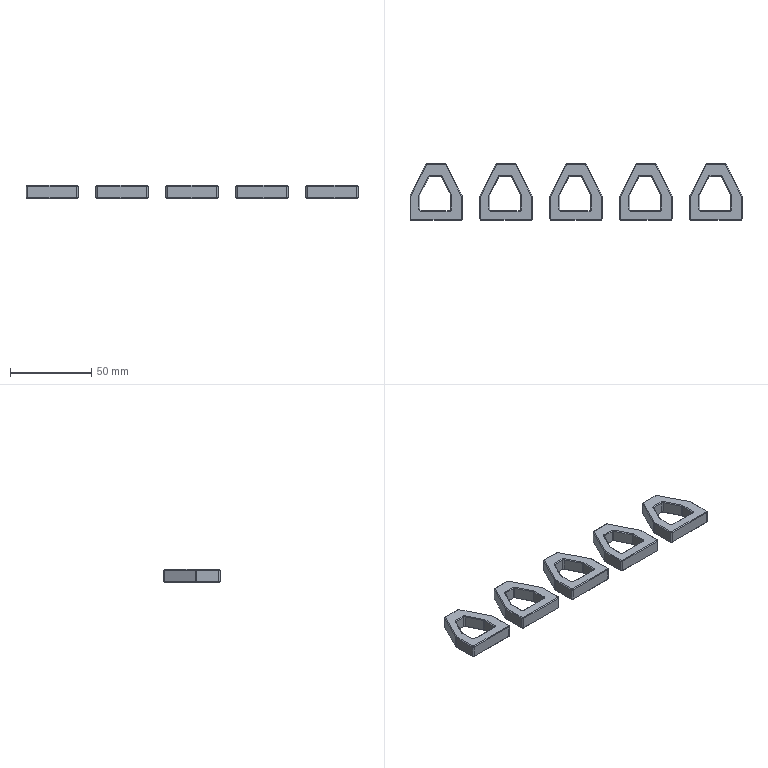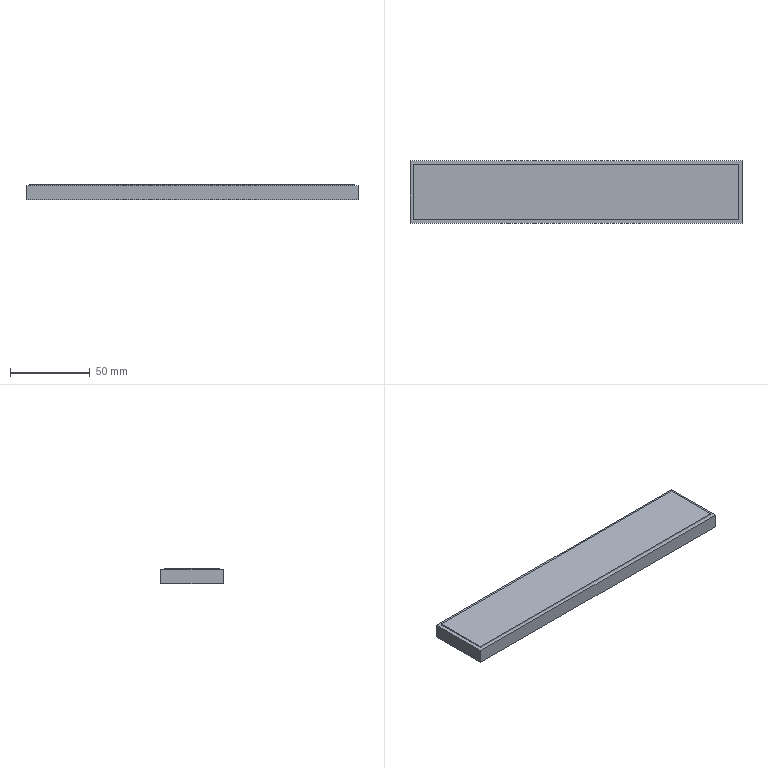CAM job | NX | 3-axis milling | part box 204 x 35 x 8 mm | stock box 208 x 39 x 10 mm
Tools:
number,name,description,diameter,corner_radius,flute_length,length,flutes
19,D80,Milling Tool-5 Parameters,80.0,0.0,50.0,75.0,2
15,D10,Milling Tool-5 Parameters,10.0,0.0,50.0,75.0,2
14,D10JING,Milling Tool-5 Parameters,10.0,0.0,50.0,75.0,2
11,D4,Milling Tool-5 Parameters,4.0,0.0,50.0,75.0,2
17,D3,Milling Tool-5 Parameters,3.0,0.0,50.0,75.0,2
16,D2,Milling Tool-5 Parameters,2.0,0.0,50.0,75.0,2
1,D6A45,Milling Tool-5 Parameters,6.0,0.0,50.0,75.0,2
Operations:
program,operation,operation_type,tool,method,geometry_group,spindle_rpm,surface_speed,feed_per_tooth,feed_cut,feed_plunge,cut_length_mm,path_length_mm,cut_time_min,machine_time_min
1,FLOOR_WALL,VolumeBased25DMillingOperation,D80,METHOD,A,6500.0,1633.0,0.1154,1500.0,100.0,300.0,354.0,0.2,0.2054
1,ZLEVEL_PROFILE_COPY_1,ZLevelMilling,D10,METHOD,A,9500.0,298.0,0.1842,3500.0,1000.0,8731.767,10477.213,2.836,3.01
1,PLANAR_PROFILE,PlanarMilling,D10,METHOD,A,9500.0,298.0,0.1842,3500.0,100.0,2440.0,5132.0,0.6971,0.9663
1,ZLEVEL_PROFILE_COPY_1_COPY,ZLevelMilling,D10JING,METHOD,A,9500.0,298.0,0.0632,1200.0,1000.0,967.776,2493.494,0.8107,0.9633
1,ZLEVEL_PROFILE_COPY_1_COPY_1,ZLevelMilling,D4,METHOD,A,9500.0,298.0,0.0947,1800.0,1000.0,3024.927,7224.257,1.863,2.282
1,HOLE_MILLING,CylinderMilling,D3,METHOD,A,9500.0,89.0,0.0605,1150.0,100.0,1287.723,2989.856,1.12,1.29
1,ZLEVEL_PROFILE_COPY_1_COPY_1_COPY,ZLevelMilling,D2,METHOD,A,9500.0,59.0,0.0642,1220.0,1000.0,2050.113,5084.09,1.727,2.031
1,PLANAR_MILL_COPY_COPY_COPY_COPY,PlanarMilling,D6A45,METHOD,A,9500.0,179.0,0.0658,1250.0,100.0,1217.163,3503.614,0.9737,1.202
1,刀补17,CylinderMilling,D3,METHOD,A,9500.0,89.0,0.0605,1150.0,100.0,292.32,1994.452,0.2542,0.4244
2,FLOOR_WALL_COPY,VolumeBased25DMillingOperation,D80,METHOD,B,6500.0,1633.0,0.1154,1500.0,100.0,1184.0,2264.001,0.7893,0.8973
2,PLANAR_MILL_COPY_COPY_COPY_COPY_COPY,PlanarMilling,D6A45,METHOD,B,9500.0,179.0,0.0658,1250.0,100.0,989.612,1894.814,0.7917,0.8822